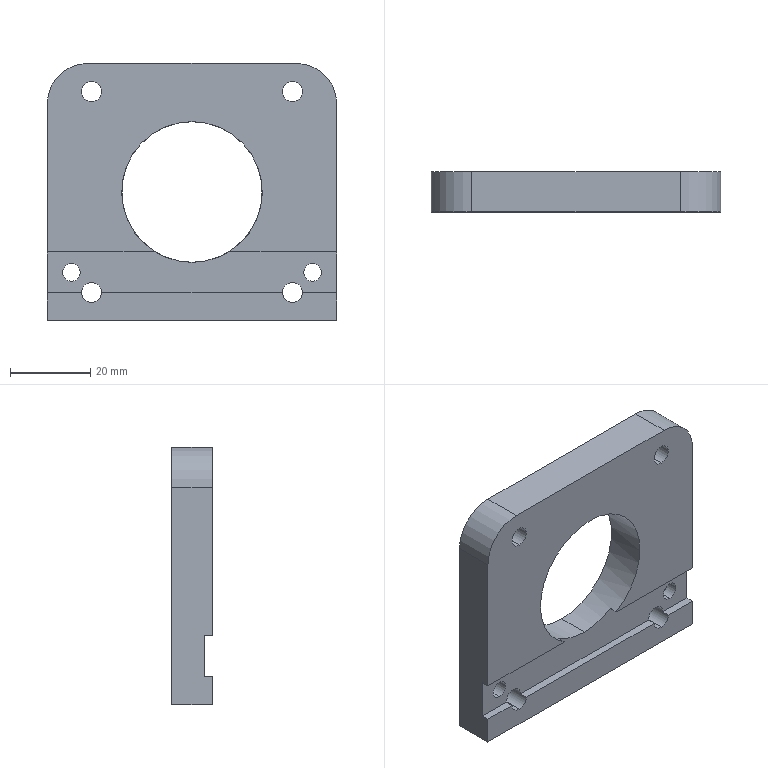Part | SolidWorks | features HoleWzd 5, ICE 5, Fillet 2, Extrusion 1 | 1 solid | 35 faces | box 72 x 10 x 64 mm | volume 33293 mm3 | cylinder 20 | plane 15 | commonest cylinder face diameters 5 x8 4.4 x4 8 x4 20 x2 35 x2
STEP:
#1=CARTESIAN_POINT('',(26.5,0.,40.5));
#2=VERTEX_POINT('',#1);
#3=CARTESIAN_POINT('',(24.001,0.,42.925));
#4=VERTEX_POINT('',#3);
#5=CARTESIAN_POINT('',(26.5,0.,43.));
#6=DIRECTION('',(0.,1.,0.));
#7=DIRECTION('',(0.,0.,1.));
#8=AXIS2_PLACEMENT_3D('',#5,#6,#7);
#9=CIRCLE('',#8,2.5);
#10=EDGE_CURVE('',#2,#4,#9,.T.);
#11=ORIENTED_EDGE('',*,*,#10,.F.);
#12=CARTESIAN_POINT('',(26.5,10.,40.5));
#13=VERTEX_POINT('',#12);
#14=CARTESIAN_POINT('',(26.5,10.,40.5));
#15=DIRECTION('',(0.,1.,0.));
#16=VECTOR('',#15,1000.);
#17=LINE('',#14,#16);
#18=EDGE_CURVE('',#2,#13,#17,.T.);
#19=ORIENTED_EDGE('',*,*,#18,.T.);
#20=CARTESIAN_POINT('',(26.5,10.,45.5));
#21=VERTEX_POINT('',#20);
#22=CARTESIAN_POINT('',(26.5,10.,43.));
#23=DIRECTION('',(0.,1.,0.));
#24=DIRECTION('',(0.,0.,1.));
#25=AXIS2_PLACEMENT_3D('',#22,#23,#24);
#26=CIRCLE('',#25,2.5);
#27=EDGE_CURVE('',#13,#21,#26,.T.);
#28=ORIENTED_EDGE('',*,*,#27,.T.);
#29=CARTESIAN_POINT('',(26.5,2.,45.5));
#30=VERTEX_POINT('',#29);
#31=CARTESIAN_POINT('',(26.5,10.,45.5));
#32=DIRECTION('',(0.,1.,0.));
#33=VECTOR('',#32,1000.);
#34=LINE('',#31,#33);
#35=EDGE_CURVE('',#30,#21,#34,.T.);
#36=ORIENTED_EDGE('',*,*,#35,.F.);
#37=CARTESIAN_POINT('',(24.001,2.,42.925));
#38=VERTEX_POINT('',#37);
#39=CARTESIAN_POINT('',(26.5,2.,43.));
#40=DIRECTION('',(0.,1.,0.));
#41=DIRECTION('',(0.,0.,-1.));
#42=AXIS2_PLACEMENT_3D('',#39,#40,#41);
#43=CIRCLE('',#42,2.5);
#44=EDGE_CURVE('',#38,#30,#43,.T.);
#45=ORIENTED_EDGE('',*,*,#44,.F.);
#46=CARTESIAN_POINT('',(24.001,10.,42.925));
#47=DIRECTION('',(0.,-1.,0.));
#48=VECTOR('',#47,1000.);
#49=LINE('',#46,#48);
#50=EDGE_CURVE('',#38,#4,#49,.T.);
#51=ORIENTED_EDGE('',*,*,#50,.T.);
#52=EDGE_LOOP('',(#11,#19,#28,#36,#45,#51));
#53=FACE_OUTER_BOUND('',#52,.T.);
#54=CARTESIAN_POINT('',(26.5,10.,43.));
#55=DIRECTION('',(0.,1.,0.));
#56=DIRECTION('',(0.,0.,1.));
#57=AXIS2_PLACEMENT_3D('',#54,#55,#56);
#58=CYLINDRICAL_SURFACE('',#57,2.5);
#59=ADVANCED_FACE('',(#53),#58,.F.);
#60=CARTESIAN_POINT('',(26.5,0.,90.5));
#61=VERTEX_POINT('',#60);
#62=CARTESIAN_POINT('',(26.5,0.,95.5));
#63=VERTEX_POINT('',#62);
#64=CARTESIAN_POINT('',(26.5,0.,93.));
#65=DIRECTION('',(0.,1.,0.));
#66=DIRECTION('',(0.,0.,1.));
#67=AXIS2_PLACEMENT_3D('',#64,#65,#66);
#68=CIRCLE('',#67,2.5);
#69=EDGE_CURVE('',#61,#63,#68,.T.);
#70=ORIENTED_EDGE('',*,*,#69,.F.);
#71=CARTESIAN_POINT('',(26.5,10.,90.5));
#72=VERTEX_POINT('',#71);
#73=CARTESIAN_POINT('',(26.5,10.,90.5));
#74=DIRECTION('',(0.,1.,0.));
#75=VECTOR('',#74,1000.);
#76=LINE('',#73,#75);
#77=EDGE_CURVE('',#61,#72,#76,.T.);
#78=ORIENTED_EDGE('',*,*,#77,.T.);
#79=CARTESIAN_POINT('',(26.5,10.,95.5));
#80=VERTEX_POINT('',#79);
#81=CARTESIAN_POINT('',(26.5,10.,93.));
#82=DIRECTION('',(0.,1.,0.));
#83=DIRECTION('',(0.,0.,1.));
#84=AXIS2_PLACEMENT_3D('',#81,#82,#83);
#85=CIRCLE('',#84,2.5);
#86=EDGE_CURVE('',#72,#80,#85,.T.);
#87=ORIENTED_EDGE('',*,*,#86,.T.);
#88=CARTESIAN_POINT('',(26.5,10.,95.5));
#89=DIRECTION('',(0.,1.,0.));
#90=VECTOR('',#89,1000.);
#91=LINE('',#88,#90);
#92=EDGE_CURVE('',#63,#80,#91,.T.);
#93=ORIENTED_EDGE('',*,*,#92,.F.);
#94=EDGE_LOOP('',(#70,#78,#87,#93));
#95=FACE_OUTER_BOUND('',#94,.T.);
#96=CARTESIAN_POINT('',(26.5,10.,93.));
#97=DIRECTION('',(0.,1.,0.));
#98=DIRECTION('',(0.,0.,1.));
#99=AXIS2_PLACEMENT_3D('',#96,#97,#98);
#100=CYLINDRICAL_SURFACE('',#99,2.5);
#101=ADVANCED_FACE('',(#95),#100,.F.);
#102=CARTESIAN_POINT('',(76.5,0.,90.5));
#103=VERTEX_POINT('',#102);
#104=CARTESIAN_POINT('',(76.5,0.,95.5));
#105=VERTEX_POINT('',#104);
#106=CARTESIAN_POINT('',(76.5,0.,93.));
#107=DIRECTION('',(0.,1.,0.));
#108=DIRECTION('',(0.,0.,1.));
#109=AXIS2_PLACEMENT_3D('',#106,#107,#108);
#110=CIRCLE('',#109,2.5);
#111=EDGE_CURVE('',#103,#105,#110,.T.);
#112=ORIENTED_EDGE('',*,*,#111,.F.);
#113=CARTESIAN_POINT('',(76.5,10.,90.5));
#114=VERTEX_POINT('',#113);
#115=CARTESIAN_POINT('',(76.5,10.,90.5));
#116=DIRECTION('',(0.,1.,0.));
#117=VECTOR('',#116,1000.);
#118=LINE('',#115,#117);
#119=EDGE_CURVE('',#103,#114,#118,.T.);
#120=ORIENTED_EDGE('',*,*,#119,.T.);
#121=CARTESIAN_POINT('',(76.5,10.,95.5));
#122=VERTEX_POINT('',#121);
#123=CARTESIAN_POINT('',(76.5,10.,93.));
#124=DIRECTION('',(0.,1.,0.));
#125=DIRECTION('',(0.,0.,1.));
#126=AXIS2_PLACEMENT_3D('',#123,#124,#125);
#127=CIRCLE('',#126,2.5);
#128=EDGE_CURVE('',#114,#122,#127,.T.);
#129=ORIENTED_EDGE('',*,*,#128,.T.);
#130=CARTESIAN_POINT('',(76.5,10.,95.5));
#131=DIRECTION('',(0.,1.,0.));
#132=VECTOR('',#131,1000.);
#133=LINE('',#130,#132);
#134=EDGE_CURVE('',#105,#122,#133,.T.);
#135=ORIENTED_EDGE('',*,*,#134,.F.);
#136=EDGE_LOOP('',(#112,#120,#129,#135));
#137=FACE_OUTER_BOUND('',#136,.T.);
#138=CARTESIAN_POINT('',(76.5,10.,93.));
#139=DIRECTION('',(0.,1.,0.));
#140=DIRECTION('',(0.,0.,1.));
#141=AXIS2_PLACEMENT_3D('',#138,#139,#140);
#142=CYLINDRICAL_SURFACE('',#141,2.5);
#143=ADVANCED_FACE('',(#137),#142,.F.);
#144=CARTESIAN_POINT('',(76.5,0.,40.5));
#145=VERTEX_POINT('',#144);
#146=CARTESIAN_POINT('',(74.001,0.,42.925));
#147=VERTEX_POINT('',#146);
#148=CARTESIAN_POINT('',(76.5,0.,43.));
#149=DIRECTION('',(0.,1.,0.));
#150=DIRECTION('',(0.,0.,1.));
#151=AXIS2_PLACEMENT_3D('',#148,#149,#150);
#152=CIRCLE('',#151,2.5);
#153=EDGE_CURVE('',#145,#147,#152,.T.);
#154=ORIENTED_EDGE('',*,*,#153,.F.);
#155=CARTESIAN_POINT('',(76.5,10.,40.5));
#156=VERTEX_POINT('',#155);
#157=CARTESIAN_POINT('',(76.5,10.,40.5));
#158=DIRECTION('',(0.,1.,0.));
#159=VECTOR('',#158,1000.);
#160=LINE('',#157,#159);
#161=EDGE_CURVE('',#145,#156,#160,.T.);
#162=ORIENTED_EDGE('',*,*,#161,.T.);
#163=CARTESIAN_POINT('',(76.5,10.,45.5));
#164=VERTEX_POINT('',#163);
#165=CARTESIAN_POINT('',(76.5,10.,43.));
#166=DIRECTION('',(0.,1.,0.));
#167=DIRECTION('',(0.,0.,1.));
#168=AXIS2_PLACEMENT_3D('',#165,#166,#167);
#169=CIRCLE('',#168,2.5);
#170=EDGE_CURVE('',#156,#164,#169,.T.);
#171=ORIENTED_EDGE('',*,*,#170,.T.);
#172=CARTESIAN_POINT('',(76.5,2.,45.5));
#173=VERTEX_POINT('',#172);
#174=CARTESIAN_POINT('',(76.5,10.,45.5));
#175=DIRECTION('',(0.,1.,0.));
#176=VECTOR('',#175,1000.);
#177=LINE('',#174,#176);
#178=EDGE_CURVE('',#173,#164,#177,.T.);
#179=ORIENTED_EDGE('',*,*,#178,.F.);
#180=CARTESIAN_POINT('',(74.001,2.,42.925));
#181=VERTEX_POINT('',#180);
#182=CARTESIAN_POINT('',(76.5,2.,43.));
#183=DIRECTION('',(0.,1.,0.));
#184=DIRECTION('',(0.,0.,-1.));
#185=AXIS2_PLACEMENT_3D('',#182,#183,#184);
#186=CIRCLE('',#185,2.5);
#187=EDGE_CURVE('',#181,#173,#186,.T.);
#188=ORIENTED_EDGE('',*,*,#187,.F.);
#189=CARTESIAN_POINT('',(74.001,10.,42.925));
#190=DIRECTION('',(0.,-1.,0.));
#191=VECTOR('',#190,1000.);
#192=LINE('',#189,#191);
#193=EDGE_CURVE('',#181,#147,#192,.T.);
#194=ORIENTED_EDGE('',*,*,#193,.T.);
#195=EDGE_LOOP('',(#154,#162,#171,#179,#188,#194));
#196=FACE_OUTER_BOUND('',#195,.T.);
#197=CARTESIAN_POINT('',(76.5,10.,43.));
#198=DIRECTION('',(0.,1.,0.));
#199=DIRECTION('',(0.,0.,1.));
#200=AXIS2_PLACEMENT_3D('',#197,#198,#199);
#201=CYLINDRICAL_SURFACE('',#200,2.5);
#202=ADVANCED_FACE('',(#196),#201,.F.);
#203=CARTESIAN_POINT('',(21.5,5.,44.));
#204=VERTEX_POINT('',#203);
#205=CARTESIAN_POINT('',(21.5,5.,52.));
#206=VERTEX_POINT('',#205);
#207=CARTESIAN_POINT('',(21.5,5.,48.));
#208=DIRECTION('',(0.,1.,0.));
#209=DIRECTION('',(0.,0.,1.));
#210=AXIS2_PLACEMENT_3D('',#207,#208,#209);
#211=CIRCLE('',#210,4.);
#212=EDGE_CURVE('',#204,#206,#211,.T.);
#213=ORIENTED_EDGE('',*,*,#212,.F.);
#214=CARTESIAN_POINT('',(21.5,10.,44.));
#215=VERTEX_POINT('',#214);
#216=CARTESIAN_POINT('',(21.5,10.,44.));
#217=DIRECTION('',(0.,1.,0.));
#218=VECTOR('',#217,1000.);
#219=LINE('',#216,#218);
#220=EDGE_CURVE('',#204,#215,#219,.T.);
#221=ORIENTED_EDGE('',*,*,#220,.T.);
#222=CARTESIAN_POINT('',(21.5,10.,52.));
#223=VERTEX_POINT('',#222);
#224=CARTESIAN_POINT('',(21.5,10.,48.));
#225=DIRECTION('',(0.,1.,0.));
#226=DIRECTION('',(0.,0.,1.));
#227=AXIS2_PLACEMENT_3D('',#224,#225,#226);
#228=CIRCLE('',#227,4.);
#229=EDGE_CURVE('',#215,#223,#228,.T.);
#230=ORIENTED_EDGE('',*,*,#229,.T.);
#231=CARTESIAN_POINT('',(21.5,10.,52.));
#232=DIRECTION('',(0.,1.,0.));
#233=VECTOR('',#232,1000.);
#234=LINE('',#231,#233);
#235=EDGE_CURVE('',#206,#223,#234,.T.);
#236=ORIENTED_EDGE('',*,*,#235,.F.);
#237=EDGE_LOOP('',(#213,#221,#230,#236));
#238=FACE_OUTER_BOUND('',#237,.T.);
#239=CARTESIAN_POINT('',(21.5,10.,48.));
#240=DIRECTION('',(0.,1.,0.));
#241=DIRECTION('',(0.,0.,1.));
#242=AXIS2_PLACEMENT_3D('',#239,#240,#241);
#243=CYLINDRICAL_SURFACE('',#242,4.);
#244=ADVANCED_FACE('',(#238),#243,.F.);
#245=CARTESIAN_POINT('',(81.5,5.,44.));
#246=VERTEX_POINT('',#245);
#247=CARTESIAN_POINT('',(81.5,5.,52.));
#248=VERTEX_POINT('',#247);
#249=CARTESIAN_POINT('',(81.5,5.,48.));
#250=DIRECTION('',(0.,1.,0.));
#251=DIRECTION('',(0.,0.,1.));
#252=AXIS2_PLACEMENT_3D('',#249,#250,#251);
#253=CIRCLE('',#252,4.);
#254=EDGE_CURVE('',#246,#248,#253,.T.);
#255=ORIENTED_EDGE('',*,*,#254,.F.);
#256=CARTESIAN_POINT('',(81.5,10.,44.));
#257=VERTEX_POINT('',#256);
#258=CARTESIAN_POINT('',(81.5,10.,44.));
#259=DIRECTION('',(0.,1.,0.));
#260=VECTOR('',#259,1000.);
#261=LINE('',#258,#260);
#262=EDGE_CURVE('',#246,#257,#261,.T.);
#263=ORIENTED_EDGE('',*,*,#262,.T.);
#264=CARTESIAN_POINT('',(81.5,10.,52.));
#265=VERTEX_POINT('',#264);
#266=CARTESIAN_POINT('',(81.5,10.,48.));
#267=DIRECTION('',(0.,1.,0.));
#268=DIRECTION('',(0.,0.,1.));
#269=AXIS2_PLACEMENT_3D('',#266,#267,#268);
#270=CIRCLE('',#269,4.);
#271=EDGE_CURVE('',#257,#265,#270,.T.);
#272=ORIENTED_EDGE('',*,*,#271,.T.);
#273=CARTESIAN_POINT('',(81.5,10.,52.));
#274=DIRECTION('',(0.,1.,0.));
#275=VECTOR('',#274,1000.);
#276=LINE('',#273,#275);
#277=EDGE_CURVE('',#248,#265,#276,.T.);
#278=ORIENTED_EDGE('',*,*,#277,.F.);
#279=EDGE_LOOP('',(#255,#263,#272,#278));
#280=FACE_OUTER_BOUND('',#279,.T.);
#281=CARTESIAN_POINT('',(81.5,10.,48.));
#282=DIRECTION('',(0.,1.,0.));
#283=DIRECTION('',(0.,0.,1.));
#284=AXIS2_PLACEMENT_3D('',#281,#282,#283);
#285=CYLINDRICAL_SURFACE('',#284,4.);
#286=ADVANCED_FACE('',(#280),#285,.F.);
#287=CARTESIAN_POINT('',(51.5,2.,50.5));
#288=VERTEX_POINT('',#287);
#289=CARTESIAN_POINT('',(42.362,2.,53.075));
#290=VERTEX_POINT('',#289);
#291=CARTESIAN_POINT('',(51.5,2.,68.));
#292=DIRECTION('',(0.,1.,0.));
#293=DIRECTION('',(0.,0.,-1.));
#294=AXIS2_PLACEMENT_3D('',#291,#292,#293);
#295=CIRCLE('',#294,17.5);
#296=EDGE_CURVE('',#288,#290,#295,.T.);
#297=ORIENTED_EDGE('',*,*,#296,.F.);
#298=CARTESIAN_POINT('',(51.5,10.,50.5));
#299=VERTEX_POINT('',#298);
#300=CARTESIAN_POINT('',(51.5,0.,50.5));
#301=DIRECTION('',(0.,1.,0.));
#302=VECTOR('',#301,1000.);
#303=LINE('',#300,#302);
#304=EDGE_CURVE('',#288,#299,#303,.T.);
#305=ORIENTED_EDGE('',*,*,#304,.T.);
#306=CARTESIAN_POINT('',(51.5,10.,85.5));
#307=VERTEX_POINT('',#306);
#308=CARTESIAN_POINT('',(51.5,10.,68.));
#309=DIRECTION('',(0.,1.,0.));
#310=DIRECTION('',(0.,0.,1.));
#311=AXIS2_PLACEMENT_3D('',#308,#309,#310);
#312=CIRCLE('',#311,17.5);
#313=EDGE_CURVE('',#299,#307,#312,.T.);
#314=ORIENTED_EDGE('',*,*,#313,.T.);
#315=CARTESIAN_POINT('',(51.5,0.,85.5));
#316=VERTEX_POINT('',#315);
#317=CARTESIAN_POINT('',(51.5,0.,85.5));
#318=DIRECTION('',(0.,1.,0.));
#319=VECTOR('',#318,1000.);
#320=LINE('',#317,#319);
#321=EDGE_CURVE('',#316,#307,#320,.T.);
#322=ORIENTED_EDGE('',*,*,#321,.F.);
#323=CARTESIAN_POINT('',(42.362,0.,53.075));
#324=VERTEX_POINT('',#323);
#325=CARTESIAN_POINT('',(51.5,0.,68.));
#326=DIRECTION('',(0.,1.,0.));
#327=DIRECTION('',(0.,0.,1.));
#328=AXIS2_PLACEMENT_3D('',#325,#326,#327);
#329=CIRCLE('',#328,17.5);
#330=EDGE_CURVE('',#324,#316,#329,.T.);
#331=ORIENTED_EDGE('',*,*,#330,.F.);
#332=CARTESIAN_POINT('',(42.362,0.,53.075));
#333=DIRECTION('',(0.,1.,0.));
#334=VECTOR('',#333,1000.);
#335=LINE('',#332,#334);
#336=EDGE_CURVE('',#324,#290,#335,.T.);
#337=ORIENTED_EDGE('',*,*,#336,.T.);
#338=EDGE_LOOP('',(#297,#305,#314,#322,#331,#337));
#339=FACE_OUTER_BOUND('',#338,.T.);
#340=CARTESIAN_POINT('',(51.5,0.,68.));
#341=DIRECTION('',(0.,1.,0.));
#342=DIRECTION('',(0.,0.,1.));
#343=AXIS2_PLACEMENT_3D('',#340,#341,#342);
#344=CYLINDRICAL_SURFACE('',#343,17.5);
#345=ADVANCED_FACE('',(#339),#344,.F.);
#346=CARTESIAN_POINT('',(21.5,2.,45.8));
#347=VERTEX_POINT('',#346);
#348=CARTESIAN_POINT('',(21.5,2.,50.2));
#349=VERTEX_POINT('',#348);
#350=CARTESIAN_POINT('',(21.5,2.,48.));
#351=DIRECTION('',(0.,1.,0.));
#352=DIRECTION('',(0.,0.,-1.));
#353=AXIS2_PLACEMENT_3D('',#350,#351,#352);
#354=CIRCLE('',#353,2.2);
#355=EDGE_CURVE('',#347,#349,#354,.T.);
#356=ORIENTED_EDGE('',*,*,#355,.F.);
#357=CARTESIAN_POINT('',(21.5,5.,45.8));
#358=VERTEX_POINT('',#357);
#359=CARTESIAN_POINT('',(21.5,10.,45.8));
#360=DIRECTION('',(0.,1.,0.));
#361=VECTOR('',#360,1000.);
#362=LINE('',#359,#361);
#363=EDGE_CURVE('',#347,#358,#362,.T.);
#364=ORIENTED_EDGE('',*,*,#363,.T.);
#365=CARTESIAN_POINT('',(21.5,5.,50.2));
#366=VERTEX_POINT('',#365);
#367=CARTESIAN_POINT('',(21.5,5.,48.));
#368=DIRECTION('',(0.,1.,0.));
#369=DIRECTION('',(0.,0.,1.));
#370=AXIS2_PLACEMENT_3D('',#367,#368,#369);
#371=CIRCLE('',#370,2.2);
#372=EDGE_CURVE('',#358,#366,#371,.T.);
#373=ORIENTED_EDGE('',*,*,#372,.T.);
#374=CARTESIAN_POINT('',(21.5,10.,50.2));
#375=DIRECTION('',(0.,1.,0.));
#376=VECTOR('',#375,1000.);
#377=LINE('',#374,#376);
#378=EDGE_CURVE('',#349,#366,#377,.T.);
#379=ORIENTED_EDGE('',*,*,#378,.F.);
#380=EDGE_LOOP('',(#356,#364,#373,#379));
#381=FACE_OUTER_BOUND('',#380,.T.);
#382=CARTESIAN_POINT('',(21.5,10.,48.));
#383=DIRECTION('',(0.,1.,0.));
#384=DIRECTION('',(0.,0.,1.));
#385=AXIS2_PLACEMENT_3D('',#382,#383,#384);
#386=CYLINDRICAL_SURFACE('',#385,2.2);
#387=ADVANCED_FACE('',(#381),#386,.F.);
#388=CARTESIAN_POINT('',(81.5,2.,45.8));
#389=VERTEX_POINT('',#388);
#390=CARTESIAN_POINT('',(81.5,2.,50.2));
#391=VERTEX_POINT('',#390);
#392=CARTESIAN_POINT('',(81.5,2.,48.));
#393=DIRECTION('',(0.,1.,0.));
#394=DIRECTION('',(0.,0.,-1.));
#395=AXIS2_PLACEMENT_3D('',#392,#393,#394);
#396=CIRCLE('',#395,2.2);
#397=EDGE_CURVE('',#389,#391,#396,.T.);
#398=ORIENTED_EDGE('',*,*,#397,.F.);
#399=CARTESIAN_POINT('',(81.5,5.,45.8));
#400=VERTEX_POINT('',#399);
#401=CARTESIAN_POINT('',(81.5,10.,45.8));
#402=DIRECTION('',(0.,1.,0.));
#403=VECTOR('',#402,1000.);
#404=LINE('',#401,#403);
#405=EDGE_CURVE('',#389,#400,#404,.T.);
#406=ORIENTED_EDGE('',*,*,#405,.T.);
#407=CARTESIAN_POINT('',(81.5,5.,50.2));
#408=VERTEX_POINT('',#407);
#409=CARTESIAN_POINT('',(81.5,5.,48.));
#410=DIRECTION('',(0.,1.,0.));
#411=DIRECTION('',(0.,0.,1.));
#412=AXIS2_PLACEMENT_3D('',#409,#410,#411);
#413=CIRCLE('',#412,2.2);
#414=EDGE_CURVE('',#400,#408,#413,.T.);
#415=ORIENTED_EDGE('',*,*,#414,.T.);
#416=CARTESIAN_POINT('',(81.5,10.,50.2));
#417=DIRECTION('',(0.,1.,0.));
#418=VECTOR('',#417,1000.);
#419=LINE('',#416,#418);
#420=EDGE_CURVE('',#391,#408,#419,.T.);
#421=ORIENTED_EDGE('',*,*,#420,.F.);
#422=EDGE_LOOP('',(#398,#406,#415,#421));
#423=FACE_OUTER_BOUND('',#422,.T.);
#424=CARTESIAN_POINT('',(81.5,10.,48.));
#425=DIRECTION('',(0.,1.,0.));
#426=DIRECTION('',(0.,0.,1.));
#427=AXIS2_PLACEMENT_3D('',#424,#425,#426);
#428=CYLINDRICAL_SURFACE('',#427,2.2);
#429=ADVANCED_FACE('',(#423),#428,.F.);
#430=CARTESIAN_POINT('',(15.5,0.,42.925));
#431=VERTEX_POINT('',#430);
#432=CARTESIAN_POINT('',(-50.34,0.,42.925));
#433=DIRECTION('',(1.,0.,0.));
#434=VECTOR('',#433,1000.);
#435=LINE('',#432,#434);
#436=EDGE_CURVE('',#431,#4,#435,.T.);
#437=ORIENTED_EDGE('',*,*,#436,.F.);
#438=CARTESIAN_POINT('',(15.5,0.,36.));
#439=VERTEX_POINT('',#438);
#440=CARTESIAN_POINT('',(15.5,0.,100.));
#441=DIRECTION('',(0.,0.,-1.));
#442=VECTOR('',#441,1000.);
#443=LINE('',#440,#442);
#444=EDGE_CURVE('',#431,#439,#443,.T.);
#445=ORIENTED_EDGE('',*,*,#444,.T.);
#446=CARTESIAN_POINT('',(87.5,0.,36.));
#447=VERTEX_POINT('',#446);
#448=CARTESIAN_POINT('',(0.,0.,36.));
#449=DIRECTION('',(-1.,0.,0.));
#450=VECTOR('',#449,1000.);
#451=LINE('',#448,#450);
#452=EDGE_CURVE('',#447,#439,#451,.T.);
#453=ORIENTED_EDGE('',*,*,#452,.F.);
#454=CARTESIAN_POINT('',(87.5,0.,42.925));
#455=VERTEX_POINT('',#454);
#456=CARTESIAN_POINT('',(87.5,0.,100.));
#457=DIRECTION('',(0.,0.,1.));
#458=VECTOR('',#457,1000.);
#459=LINE('',#456,#458);
#460=EDGE_CURVE('',#447,#455,#459,.T.);
#461=ORIENTED_EDGE('',*,*,#460,.T.);
#462=CARTESIAN_POINT('',(78.999,0.,42.925));
#463=VERTEX_POINT('',#462);
#464=CARTESIAN_POINT('',(-50.34,0.,42.925));
#465=DIRECTION('',(1.,0.,0.));
#466=VECTOR('',#465,1000.);
#467=LINE('',#464,#466);
#468=EDGE_CURVE('',#463,#455,#467,.T.);
#469=ORIENTED_EDGE('',*,*,#468,.F.);
#470=CARTESIAN_POINT('',(76.5,0.,43.));
#471=DIRECTION('',(0.,1.,0.));
#472=DIRECTION('',(0.,0.,1.));
#473=AXIS2_PLACEMENT_3D('',#470,#471,#472);
#474=CIRCLE('',#473,2.5);
#475=EDGE_CURVE('',#463,#145,#474,.T.);
#476=ORIENTED_EDGE('',*,*,#475,.T.);
#477=ORIENTED_EDGE('',*,*,#153,.T.);
#478=CARTESIAN_POINT('',(28.999,0.,42.925));
#479=VERTEX_POINT('',#478);
#480=CARTESIAN_POINT('',(-50.34,0.,42.925));
#481=DIRECTION('',(1.,0.,0.));
#482=VECTOR('',#481,1000.);
#483=LINE('',#480,#482);
#484=EDGE_CURVE('',#479,#147,#483,.T.);
#485=ORIENTED_EDGE('',*,*,#484,.F.);
#486=CARTESIAN_POINT('',(26.5,0.,43.));
#487=DIRECTION('',(0.,1.,0.));
#488=DIRECTION('',(0.,0.,1.));
#489=AXIS2_PLACEMENT_3D('',#486,#487,#488);
#490=CIRCLE('',#489,2.5);
#491=EDGE_CURVE('',#479,#2,#490,.T.);
#492=ORIENTED_EDGE('',*,*,#491,.T.);
#493=ORIENTED_EDGE('',*,*,#10,.T.);
#494=EDGE_LOOP('',(#437,#445,#453,#461,#469,#476,#477,#485,#492,#493));
#495=FACE_OUTER_BOUND('',#494,.T.);
#496=CARTESIAN_POINT('',(0.,0.,0.));
#497=DIRECTION('',(0.,-1.,0.));
#498=DIRECTION('',(0.,0.,-1.));
#499=AXIS2_PLACEMENT_3D('',#496,#497,#498);
#500=PLANE('',#499);
#501=ADVANCED_FACE('',(#495),#500,.T.);
#502=ORIENTED_EDGE('',*,*,#405,.F.);
#503=CARTESIAN_POINT('',(81.5,2.,48.));
#504=DIRECTION('',(0.,1.,0.));
#505=DIRECTION('',(0.,0.,-1.));
#506=AXIS2_PLACEMENT_3D('',#503,#504,#505);
#507=CIRCLE('',#506,2.2);
#508=EDGE_CURVE('',#391,#389,#507,.T.);
#509=ORIENTED_EDGE('',*,*,#508,.F.);
#510=ORIENTED_EDGE('',*,*,#420,.T.);
#511=CARTESIAN_POINT('',(81.5,5.,48.));
#512=DIRECTION('',(0.,1.,0.));
#513=DIRECTION('',(0.,0.,1.));
#514=AXIS2_PLACEMENT_3D('',#511,#512,#513);
#515=CIRCLE('',#514,2.2);
#516=EDGE_CURVE('',#408,#400,#515,.T.);
#517=ORIENTED_EDGE('',*,*,#516,.T.);
#518=EDGE_LOOP('',(#502,#509,#510,#517));
#519=FACE_OUTER_BOUND('',#518,.T.);
#520=CARTESIAN_POINT('',(81.5,10.,48.));
#521=DIRECTION('',(0.,1.,0.));
#522=DIRECTION('',(0.,0.,1.));
#523=AXIS2_PLACEMENT_3D('',#520,#521,#522);
#524=CYLINDRICAL_SURFACE('',#523,2.2);
#525=ADVANCED_FACE('',(#519),#524,.F.);
#526=ORIENTED_EDGE('',*,*,#363,.F.);
#527=CARTESIAN_POINT('',(21.5,2.,48.));
#528=DIRECTION('',(0.,1.,0.));
#529=DIRECTION('',(0.,0.,-1.));
#530=AXIS2_PLACEMENT_3D('',#527,#528,#529);
#531=CIRCLE('',#530,2.2);
#532=EDGE_CURVE('',#349,#347,#531,.T.);
#533=ORIENTED_EDGE('',*,*,#532,.F.);
#534=ORIENTED_EDGE('',*,*,#378,.T.);
#535=CARTESIAN_POINT('',(21.5,5.,48.));
#536=DIRECTION('',(0.,1.,0.));
#537=DIRECTION('',(0.,0.,1.));
#538=AXIS2_PLACEMENT_3D('',#535,#536,#537);
#539=CIRCLE('',#538,2.2);
#540=EDGE_CURVE('',#366,#358,#539,.T.);
#541=ORIENTED_EDGE('',*,*,#540,.T.);
#542=EDGE_LOOP('',(#526,#533,#534,#541));
#543=FACE_OUTER_BOUND('',#542,.T.);
#544=CARTESIAN_POINT('',(21.5,10.,48.));
#545=DIRECTION('',(0.,1.,0.));
#546=DIRECTION('',(0.,0.,1.));
#547=AXIS2_PLACEMENT_3D('',#544,#545,#546);
#548=CYLINDRICAL_SURFACE('',#547,2.2);
#549=ADVANCED_FACE('',(#543),#548,.F.);
#550=CARTESIAN_POINT('',(25.5,10.,100.));
#551=VERTEX_POINT('',#550);
#552=CARTESIAN_POINT('',(77.5,10.,100.));
#553=VERTEX_POINT('',#552);
#554=CARTESIAN_POINT('',(103.,10.,100.));
#555=DIRECTION('',(1.,0.,0.));
#556=VECTOR('',#555,1000.);
#557=LINE('',#554,#556);
#558=EDGE_CURVE('',#551,#553,#557,.T.);
#559=ORIENTED_EDGE('',*,*,#558,.F.);
#560=CARTESIAN_POINT('',(25.5,0.,100.));
#561=VERTEX_POINT('',#560);
#562=CARTESIAN_POINT('',(25.5,10.,100.));
#563=DIRECTION('',(0.,-1.,0.));
#564=VECTOR('',#563,1000.);
#565=LINE('',#562,#564);
#566=EDGE_CURVE('',#551,#561,#565,.T.);
#567=ORIENTED_EDGE('',*,*,#566,.T.);
#568=CARTESIAN_POINT('',(77.5,0.,100.));
#569=VERTEX_POINT('',#568);
#570=CARTESIAN_POINT('',(103.,0.,100.));
#571=DIRECTION('',(1.,0.,0.));
#572=VECTOR('',#571,1000.);
#573=LINE('',#570,#572);
#574=EDGE_CURVE('',#561,#569,#573,.T.);
#575=ORIENTED_EDGE('',*,*,#574,.T.);
#576=CARTESIAN_POINT('',(77.5,10.,100.));
#577=DIRECTION('',(0.,1.,0.));
#578=VECTOR('',#577,1000.);
#579=LINE('',#576,#578);
#580=EDGE_CURVE('',#569,#553,#579,.T.);
#581=ORIENTED_EDGE('',*,*,#580,.T.);
#582=EDGE_LOOP('',(#559,#567,#575,#581));
#583=FACE_OUTER_BOUND('',#582,.T.);
#584=CARTESIAN_POINT('',(103.,10.,100.));
#585=DIRECTION('',(0.,0.,-1.));
#586=DIRECTION('',(-1.,0.,0.));
#587=AXIS2_PLACEMENT_3D('',#584,#585,#586);
#588=PLANE('',#587);
#589=ADVANCED_FACE('',(#583),#588,.F.);
#590=CARTESIAN_POINT('',(26.5,10.,43.));
#591=DIRECTION('',(0.,1.,0.));
#592=DIRECTION('',(0.,0.,1.));
#593=AXIS2_PLACEMENT_3D('',#590,#591,#592);
#594=CIRCLE('',#593,2.5);
#595=EDGE_CURVE('',#21,#13,#594,.T.);
#596=ORIENTED_EDGE('',*,*,#595,.F.);
#597=ORIENTED_EDGE('',*,*,#27,.F.);
#598=EDGE_LOOP('',(#596,#597));
#599=FACE_BOUND('',#598,.T.);
#600=CARTESIAN_POINT('',(26.5,10.,93.));
#601=DIRECTION('',(0.,1.,0.));
#602=DIRECTION('',(0.,0.,1.));
#603=AXIS2_PLACEMENT_3D('',#600,#601,#602);
#604=CIRCLE('',#603,2.5);
#605=EDGE_CURVE('',#80,#72,#604,.T.);
#606=ORIENTED_EDGE('',*,*,#605,.F.);
#607=ORIENTED_EDGE('',*,*,#86,.F.);
#608=EDGE_LOOP('',(#606,#607));
#609=FACE_BOUND('',#608,.T.);
#610=CARTESIAN_POINT('',(76.5,10.,93.));
#611=DIRECTION('',(0.,1.,0.));
#612=DIRECTION('',(0.,0.,1.));
#613=AXIS2_PLACEMENT_3D('',#610,#611,#612);
#614=CIRCLE('',#613,2.5);
#615=EDGE_CURVE('',#122,#114,#614,.T.);
#616=ORIENTED_EDGE('',*,*,#615,.F.);
#617=ORIENTED_EDGE('',*,*,#128,.F.);
#618=EDGE_LOOP('',(#616,#617));
#619=FACE_BOUND('',#618,.T.);
#620=CARTESIAN_POINT('',(76.5,10.,43.));
#621=DIRECTION('',(0.,1.,0.));
#622=DIRECTION('',(0.,0.,1.));
#623=AXIS2_PLACEMENT_3D('',#620,#621,#622);
#624=CIRCLE('',#623,2.5);
#625=EDGE_CURVE('',#164,#156,#624,.T.);
#626=ORIENTED_EDGE('',*,*,#625,.F.);
#627=ORIENTED_EDGE('',*,*,#170,.F.);
#628=EDGE_LOOP('',(#626,#627));
#629=FACE_BOUND('',#628,.T.);
#630=CARTESIAN_POINT('',(21.5,10.,48.));
#631=DIRECTION('',(0.,1.,0.));
#632=DIRECTION('',(0.,0.,1.));
#633=AXIS2_PLACEMENT_3D('',#630,#631,#632);
#634=CIRCLE('',#633,4.);
#635=EDGE_CURVE('',#223,#215,#634,.T.);
#636=ORIENTED_EDGE('',*,*,#635,.F.);
#637=ORIENTED_EDGE('',*,*,#229,.F.);
#638=EDGE_LOOP('',(#636,#637));
#639=FACE_BOUND('',#638,.T.);
#640=CARTESIAN_POINT('',(81.5,10.,48.));
#641=DIRECTION('',(0.,1.,0.));
#642=DIRECTION('',(0.,0.,1.));
#643=AXIS2_PLACEMENT_3D('',#640,#641,#642);
#644=CIRCLE('',#643,4.);
#645=EDGE_CURVE('',#265,#257,#644,.T.);
#646=ORIENTED_EDGE('',*,*,#645,.F.);
#647=ORIENTED_EDGE('',*,*,#271,.F.);
#648=EDGE_LOOP('',(#646,#647));
#649=FACE_BOUND('',#648,.T.);
#650=CARTESIAN_POINT('',(51.5,10.,68.));
#651=DIRECTION('',(0.,1.,0.));
#652=DIRECTION('',(0.,0.,1.));
#653=AXIS2_PLACEMENT_3D('',#650,#651,#652);
#654=CIRCLE('',#653,17.5);
#655=EDGE_CURVE('',#307,#299,#654,.T.);
#656=ORIENTED_EDGE('',*,*,#655,.F.);
#657=ORIENTED_EDGE('',*,*,#313,.F.);
#658=EDGE_LOOP('',(#656,#657));
#659=FACE_BOUND('',#658,.T.);
#660=CARTESIAN_POINT('',(87.5,10.,36.));
#661=VERTEX_POINT('',#660);
#662=CARTESIAN_POINT('',(87.5,10.,90.));
#663=VERTEX_POINT('',#662);
#664=CARTESIAN_POINT('',(87.5,10.,100.));
#665=DIRECTION('',(0.,0.,1.));
#666=VECTOR('',#665,1000.);
#667=LINE('',#664,#666);
#668=EDGE_CURVE('',#661,#663,#667,.T.);
#669=ORIENTED_EDGE('',*,*,#668,.F.);
#670=CARTESIAN_POINT('',(15.5,10.,36.));
#671=VERTEX_POINT('',#670);
#672=CARTESIAN_POINT('',(112.305,10.,36.));
#673=DIRECTION('',(1.,0.,0.));
#674=VECTOR('',#673,1000.);
#675=LINE('',#672,#674);
#676=EDGE_CURVE('',#671,#661,#675,.T.);
#677=ORIENTED_EDGE('',*,*,#676,.F.);
#678=CARTESIAN_POINT('',(15.5,10.,90.));
#679=VERTEX_POINT('',#678);
#680=CARTESIAN_POINT('',(15.5,10.,100.));
#681=DIRECTION('',(0.,0.,-1.));
#682=VECTOR('',#681,1000.);
#683=LINE('',#680,#682);
#684=EDGE_CURVE('',#679,#671,#683,.T.);
#685=ORIENTED_EDGE('',*,*,#684,.F.);
#686=CARTESIAN_POINT('',(25.5,10.,90.));
#687=DIRECTION('',(0.,1.,0.));
#688=DIRECTION('',(0.,0.,-1.));
#689=AXIS2_PLACEMENT_3D('',#686,#687,#688);
#690=CIRCLE('',#689,10.);
#691=EDGE_CURVE('',#679,#551,#690,.T.);
#692=ORIENTED_EDGE('',*,*,#691,.T.);
#693=ORIENTED_EDGE('',*,*,#558,.T.);
#694=CARTESIAN_POINT('',(77.5,10.,90.));
#695=DIRECTION('',(0.,1.,0.));
#696=DIRECTION('',(0.,0.,-1.));
#697=AXIS2_PLACEMENT_3D('',#694,#695,#696);
#698=CIRCLE('',#697,10.);
#699=EDGE_CURVE('',#553,#663,#698,.T.);
#700=ORIENTED_EDGE('',*,*,#699,.T.);
#701=EDGE_LOOP('',(#669,#677,#685,#692,#693,#700));
#702=FACE_OUTER_BOUND('',#701,.T.);
#703=CARTESIAN_POINT('',(0.,10.,0.));
#704=DIRECTION('',(0.,-1.,0.));
#705=DIRECTION('',(0.,0.,-1.));
#706=AXIS2_PLACEMENT_3D('',#703,#704,#705);
#707=PLANE('',#706);
#708=ADVANCED_FACE('',(#599,#609,#619,#629,#639,#649,#659,#702),#707,.F.);
#709=CARTESIAN_POINT('',(87.5,0.,53.075));
#710=VERTEX_POINT('',#709);
#711=CARTESIAN_POINT('',(60.638,0.,53.075));
#712=VERTEX_POINT('',#711);
#713=CARTESIAN_POINT('',(-50.34,0.,53.075));
#714=DIRECTION('',(-1.,0.,0.));
#715=VECTOR('',#714,1000.);
#716=LINE('',#713,#715);
#717=EDGE_CURVE('',#710,#712,#716,.T.);
#718=ORIENTED_EDGE('',*,*,#717,.F.);
#719=CARTESIAN_POINT('',(87.5,0.,90.));
#720=VERTEX_POINT('',#719);
#721=CARTESIAN_POINT('',(87.5,0.,100.));
#722=DIRECTION('',(0.,0.,1.));
#723=VECTOR('',#722,1000.);
#724=LINE('',#721,#723);
#725=EDGE_CURVE('',#710,#720,#724,.T.);
#726=ORIENTED_EDGE('',*,*,#725,.T.);
#727=CARTESIAN_POINT('',(77.5,0.,90.));
#728=DIRECTION('',(0.,-1.,0.));
#729=DIRECTION('',(0.,0.,-1.));
#730=AXIS2_PLACEMENT_3D('',#727,#728,#729);
#731=CIRCLE('',#730,10.);
#732=EDGE_CURVE('',#720,#569,#731,.T.);
#733=ORIENTED_EDGE('',*,*,#732,.T.);
#734=ORIENTED_EDGE('',*,*,#574,.F.);
#735=CARTESIAN_POINT('',(15.5,0.,90.));
#736=VERTEX_POINT('',#735);
#737=CARTESIAN_POINT('',(25.5,0.,90.));
#738=DIRECTION('',(0.,-1.,0.));
#739=DIRECTION('',(0.,0.,-1.));
#740=AXIS2_PLACEMENT_3D('',#737,#738,#739);
#741=CIRCLE('',#740,10.);
#742=EDGE_CURVE('',#561,#736,#741,.T.);
#743=ORIENTED_EDGE('',*,*,#742,.T.);
#744=CARTESIAN_POINT('',(15.5,0.,53.075));
#745=VERTEX_POINT('',#744);
#746=CARTESIAN_POINT('',(15.5,0.,100.));
#747=DIRECTION('',(0.,0.,-1.));
#748=VECTOR('',#747,1000.);
#749=LINE('',#746,#748);
#750=EDGE_CURVE('',#736,#745,#749,.T.);
#751=ORIENTED_EDGE('',*,*,#750,.T.);
#752=CARTESIAN_POINT('',(-50.34,0.,53.075));
#753=DIRECTION('',(-1.,0.,0.));
#754=VECTOR('',#753,1000.);
#755=LINE('',#752,#754);
#756=EDGE_CURVE('',#324,#745,#755,.T.);
#757=ORIENTED_EDGE('',*,*,#756,.F.);
#758=ORIENTED_EDGE('',*,*,#330,.T.);
#759=CARTESIAN_POINT('',(51.5,0.,68.));
#760=DIRECTION('',(0.,1.,0.));
#761=DIRECTION('',(0.,0.,1.));
#762=AXIS2_PLACEMENT_3D('',#759,#760,#761);
#763=CIRCLE('',#762,17.5);
#764=EDGE_CURVE('',#316,#712,#763,.T.);
#765=ORIENTED_EDGE('',*,*,#764,.T.);
#766=EDGE_LOOP('',(#718,#726,#733,#734,#743,#751,#757,#758,#765));
#767=FACE_OUTER_BOUND('',#766,.T.);
#768=CARTESIAN_POINT('',(26.5,0.,93.));
#769=DIRECTION('',(0.,1.,0.));
#770=DIRECTION('',(0.,0.,1.));
#771=AXIS2_PLACEMENT_3D('',#768,#769,#770);
#772=CIRCLE('',#771,2.5);
#773=EDGE_CURVE('',#63,#61,#772,.T.);
#774=ORIENTED_EDGE('',*,*,#773,.T.);
#775=ORIENTED_EDGE('',*,*,#69,.T.);
#776=EDGE_LOOP('',(#774,#775));
#777=FACE_BOUND('',#776,.T.);
#778=CARTESIAN_POINT('',(76.5,0.,93.));
#779=DIRECTION('',(0.,1.,0.));
#780=DIRECTION('',(0.,0.,1.));
#781=AXIS2_PLACEMENT_3D('',#778,#779,#780);
#782=CIRCLE('',#781,2.5);
#783=EDGE_CURVE('',#105,#103,#782,.T.);
#784=ORIENTED_EDGE('',*,*,#783,.T.);
#785=ORIENTED_EDGE('',*,*,#111,.T.);
#786=EDGE_LOOP('',(#784,#785));
#787=FACE_BOUND('',#786,.T.);
#788=CARTESIAN_POINT('',(0.,0.,0.));
#789=DIRECTION('',(0.,-1.,0.));
#790=DIRECTION('',(0.,0.,-1.));
#791=AXIS2_PLACEMENT_3D('',#788,#789,#790);
#792=PLANE('',#791);
#793=ADVANCED_FACE('',(#767,#777,#787),#792,.T.);
#794=ORIENTED_EDGE('',*,*,#444,.F.);
#795=CARTESIAN_POINT('',(15.5,2.,42.925));
#796=VERTEX_POINT('',#795);
#797=CARTESIAN_POINT('',(15.5,0.,42.925));
#798=DIRECTION('',(0.,1.,0.));
#799=VECTOR('',#798,1000.);
#800=LINE('',#797,#799);
#801=EDGE_CURVE('',#431,#796,#800,.T.);
#802=ORIENTED_EDGE('',*,*,#801,.T.);
#803=CARTESIAN_POINT('',(15.5,2.,53.075));
#804=VERTEX_POINT('',#803);
#805=CARTESIAN_POINT('',(15.5,2.,100.));
#806=DIRECTION('',(0.,0.,-1.));
#807=VECTOR('',#806,1000.);
#808=LINE('',#805,#807);
#809=EDGE_CURVE('',#804,#796,#808,.T.);
#810=ORIENTED_EDGE('',*,*,#809,.F.);
#811=CARTESIAN_POINT('',(15.5,0.,53.075));
#812=DIRECTION('',(0.,-1.,0.));
#813=VECTOR('',#812,1000.);
#814=LINE('',#811,#813);
#815=EDGE_CURVE('',#804,#745,#814,.T.);
#816=ORIENTED_EDGE('',*,*,#815,.T.);
#817=ORIENTED_EDGE('',*,*,#750,.F.);
#818=CARTESIAN_POINT('',(15.5,0.,90.));
#819=DIRECTION('',(0.,1.,0.));
#820=VECTOR('',#819,1000.);
#821=LINE('',#818,#820);
#822=EDGE_CURVE('',#736,#679,#821,.T.);
#823=ORIENTED_EDGE('',*,*,#822,.T.);
#824=ORIENTED_EDGE('',*,*,#684,.T.);
#825=CARTESIAN_POINT('',(15.5,0.,36.));
#826=DIRECTION('',(0.,-1.,0.));
#827=VECTOR('',#826,1000.);
#828=LINE('',#825,#827);
#829=EDGE_CURVE('',#671,#439,#828,.T.);
#830=ORIENTED_EDGE('',*,*,#829,.T.);
#831=EDGE_LOOP('',(#794,#802,#810,#816,#817,#823,#824,#830));
#832=FACE_OUTER_BOUND('',#831,.T.);
#833=CARTESIAN_POINT('',(15.5,0.,100.));
#834=DIRECTION('',(1.,0.,0.));
#835=DIRECTION('',(0.,0.,-1.));
#836=AXIS2_PLACEMENT_3D('',#833,#834,#835);
#837=PLANE('',#836);
#838=ADVANCED_FACE('',(#832),#837,.F.);
#839=CARTESIAN_POINT('',(87.5,2.,42.925));
#840=VERTEX_POINT('',#839);
#841=CARTESIAN_POINT('',(87.5,2.,53.075));
#842=VERTEX_POINT('',#841);
#843=CARTESIAN_POINT('',(87.5,2.,100.));
#844=DIRECTION('',(0.,0.,1.));
#845=VECTOR('',#844,1000.);
#846=LINE('',#843,#845);
#847=EDGE_CURVE('',#840,#842,#846,.T.);
#848=ORIENTED_EDGE('',*,*,#847,.F.);
#849=CARTESIAN_POINT('',(87.5,0.,42.925));
#850=DIRECTION('',(0.,-1.,0.));
#851=VECTOR('',#850,1000.);
#852=LINE('',#849,#851);
#853=EDGE_CURVE('',#840,#455,#852,.T.);
#854=ORIENTED_EDGE('',*,*,#853,.T.);
#855=ORIENTED_EDGE('',*,*,#460,.F.);
#856=CARTESIAN_POINT('',(87.5,0.,36.));
#857=DIRECTION('',(0.,1.,0.));
#858=VECTOR('',#857,1000.);
#859=LINE('',#856,#858);
#860=EDGE_CURVE('',#447,#661,#859,.T.);
#861=ORIENTED_EDGE('',*,*,#860,.T.);
#862=ORIENTED_EDGE('',*,*,#668,.T.);
#863=CARTESIAN_POINT('',(87.5,0.,90.));
#864=DIRECTION('',(0.,-1.,0.));
#865=VECTOR('',#864,1000.);
#866=LINE('',#863,#865);
#867=EDGE_CURVE('',#663,#720,#866,.T.);
#868=ORIENTED_EDGE('',*,*,#867,.T.);
#869=ORIENTED_EDGE('',*,*,#725,.F.);
#870=CARTESIAN_POINT('',(87.5,0.,53.075));
#871=DIRECTION('',(0.,1.,0.));
#872=VECTOR('',#871,1000.);
#873=LINE('',#870,#872);
#874=EDGE_CURVE('',#710,#842,#873,.T.);
#875=ORIENTED_EDGE('',*,*,#874,.T.);
#876=EDGE_LOOP('',(#848,#854,#855,#861,#862,#868,#869,#875));
#877=FACE_OUTER_BOUND('',#876,.T.);
#878=CARTESIAN_POINT('',(87.5,0.,100.));
#879=DIRECTION('',(-1.,0.,0.));
#880=DIRECTION('',(0.,0.,1.));
#881=AXIS2_PLACEMENT_3D('',#878,#879,#880);
#882=PLANE('',#881);
#883=ADVANCED_FACE('',(#877),#882,.F.);
#884=ORIENTED_EDGE('',*,*,#304,.F.);
#885=CARTESIAN_POINT('',(60.638,2.,53.075));
#886=VERTEX_POINT('',#885);
#887=CARTESIAN_POINT('',(51.5,2.,68.));
#888=DIRECTION('',(0.,1.,0.));
#889=DIRECTION('',(0.,0.,-1.));
#890=AXIS2_PLACEMENT_3D('',#887,#888,#889);
#891=CIRCLE('',#890,17.5);
#892=EDGE_CURVE('',#886,#288,#891,.T.);
#893=ORIENTED_EDGE('',*,*,#892,.F.);
#894=CARTESIAN_POINT('',(60.638,0.,53.075));
#895=DIRECTION('',(0.,-1.,0.));
#896=VECTOR('',#895,1000.);
#897=LINE('',#894,#896);
#898=EDGE_CURVE('',#886,#712,#897,.T.);
#899=ORIENTED_EDGE('',*,*,#898,.T.);
#900=ORIENTED_EDGE('',*,*,#764,.F.);
#901=ORIENTED_EDGE('',*,*,#321,.T.);
#902=ORIENTED_EDGE('',*,*,#655,.T.);
#903=EDGE_LOOP('',(#884,#893,#899,#900,#901,#902));
#904=FACE_OUTER_BOUND('',#903,.T.);
#905=CARTESIAN_POINT('',(51.5,0.,68.));
#906=DIRECTION('',(0.,1.,0.));
#907=DIRECTION('',(0.,0.,1.));
#908=AXIS2_PLACEMENT_3D('',#905,#906,#907);
#909=CYLINDRICAL_SURFACE('',#908,17.5);
#910=ADVANCED_FACE('',(#904),#909,.F.);
#911=ORIENTED_EDGE('',*,*,#742,.F.);
#912=ORIENTED_EDGE('',*,*,#566,.F.);
#913=ORIENTED_EDGE('',*,*,#691,.F.);
#914=ORIENTED_EDGE('',*,*,#822,.F.);
#915=EDGE_LOOP('',(#911,#912,#913,#914));
#916=FACE_OUTER_BOUND('',#915,.T.);
#917=CARTESIAN_POINT('',(25.5,0.,90.));
#918=DIRECTION('',(0.,1.,0.));
#919=DIRECTION('',(0.,0.,1.));
#920=AXIS2_PLACEMENT_3D('',#917,#918,#919);
#921=CYLINDRICAL_SURFACE('',#920,10.);
#922=ADVANCED_FACE('',(#916),#921,.T.);
#923=ORIENTED_EDGE('',*,*,#732,.F.);
#924=ORIENTED_EDGE('',*,*,#867,.F.);
#925=ORIENTED_EDGE('',*,*,#699,.F.);
#926=ORIENTED_EDGE('',*,*,#580,.F.);
#927=EDGE_LOOP('',(#923,#924,#925,#926));
#928=FACE_OUTER_BOUND('',#927,.T.);
#929=CARTESIAN_POINT('',(77.5,10.,90.));
#930=DIRECTION('',(0.,1.,0.));
#931=DIRECTION('',(0.,0.,1.));
#932=AXIS2_PLACEMENT_3D('',#929,#930,#931);
#933=CYLINDRICAL_SURFACE('',#932,10.);
#934=ADVANCED_FACE('',(#928),#933,.T.);
#935=ORIENTED_EDGE('',*,*,#676,.T.);
#936=ORIENTED_EDGE('',*,*,#860,.F.);
#937=ORIENTED_EDGE('',*,*,#452,.T.);
#938=ORIENTED_EDGE('',*,*,#829,.F.);
#939=EDGE_LOOP('',(#935,#936,#937,#938));
#940=FACE_OUTER_BOUND('',#939,.T.);
#941=CARTESIAN_POINT('',(112.305,-87.,36.));
#942=DIRECTION('',(0.,0.,1.));
#943=DIRECTION('',(1.,0.,0.));
#944=AXIS2_PLACEMENT_3D('',#941,#942,#943);
#945=PLANE('',#944);
#946=ADVANCED_FACE('',(#940),#945,.F.);
#947=ORIENTED_EDGE('',*,*,#516,.F.);
#948=ORIENTED_EDGE('',*,*,#414,.F.);
#949=EDGE_LOOP('',(#947,#948));
#950=FACE_BOUND('',#949,.T.);
#951=CARTESIAN_POINT('',(81.5,5.,48.));
#952=DIRECTION('',(0.,1.,0.));
#953=DIRECTION('',(0.,0.,1.));
#954=AXIS2_PLACEMENT_3D('',#951,#952,#953);
#955=CIRCLE('',#954,4.);
#956=EDGE_CURVE('',#248,#246,#955,.T.);
#957=ORIENTED_EDGE('',*,*,#956,.T.);
#958=ORIENTED_EDGE('',*,*,#254,.T.);
#959=EDGE_LOOP('',(#957,#958));
#960=FACE_OUTER_BOUND('',#959,.T.);
#961=CARTESIAN_POINT('',(83.7,5.,48.));
#962=DIRECTION('',(0.,-1.,0.));
#963=DIRECTION('',(0.,0.,-1.));
#964=AXIS2_PLACEMENT_3D('',#961,#962,#963);
#965=PLANE('',#964);
#966=ADVANCED_FACE('',(#950,#960),#965,.F.);
#967=ORIENTED_EDGE('',*,*,#262,.F.);
#968=ORIENTED_EDGE('',*,*,#956,.F.);
#969=ORIENTED_EDGE('',*,*,#277,.T.);
#970=ORIENTED_EDGE('',*,*,#645,.T.);
#971=EDGE_LOOP('',(#967,#968,#969,#970));
#972=FACE_OUTER_BOUND('',#971,.T.);
#973=CARTESIAN_POINT('',(81.5,10.,48.));
#974=DIRECTION('',(0.,1.,0.));
#975=DIRECTION('',(0.,0.,1.));
#976=AXIS2_PLACEMENT_3D('',#973,#974,#975);
#977=CYLINDRICAL_SURFACE('',#976,4.);
#978=ADVANCED_FACE('',(#972),#977,.F.);
#979=ORIENTED_EDGE('',*,*,#540,.F.);
#980=ORIENTED_EDGE('',*,*,#372,.F.);
#981=EDGE_LOOP('',(#979,#980));
#982=FACE_BOUND('',#981,.T.);
#983=CARTESIAN_POINT('',(21.5,5.,48.));
#984=DIRECTION('',(0.,1.,0.));
#985=DIRECTION('',(0.,0.,1.));
#986=AXIS2_PLACEMENT_3D('',#983,#984,#985);
#987=CIRCLE('',#986,4.);
#988=EDGE_CURVE('',#206,#204,#987,.T.);
#989=ORIENTED_EDGE('',*,*,#988,.T.);
#990=ORIENTED_EDGE('',*,*,#212,.T.);
#991=EDGE_LOOP('',(#989,#990));
#992=FACE_OUTER_BOUND('',#991,.T.);
#993=CARTESIAN_POINT('',(23.7,5.,48.));
#994=DIRECTION('',(0.,-1.,0.));
#995=DIRECTION('',(0.,0.,-1.));
#996=AXIS2_PLACEMENT_3D('',#993,#994,#995);
#997=PLANE('',#996);
#998=ADVANCED_FACE('',(#982,#992),#997,.F.);
#999=ORIENTED_EDGE('',*,*,#220,.F.);
#1000=ORIENTED_EDGE('',*,*,#988,.F.);
#1001=ORIENTED_EDGE('',*,*,#235,.T.);
#1002=ORIENTED_EDGE('',*,*,#635,.T.);
#1003=EDGE_LOOP('',(#999,#1000,#1001,#1002));
#1004=FACE_OUTER_BOUND('',#1003,.T.);
#1005=CARTESIAN_POINT('',(21.5,10.,48.));
#1006=DIRECTION('',(0.,1.,0.));
#1007=DIRECTION('',(0.,0.,1.));
#1008=AXIS2_PLACEMENT_3D('',#1005,#1006,#1007);
#1009=CYLINDRICAL_SURFACE('',#1008,4.);
#1010=ADVANCED_FACE('',(#1004),#1009,.F.);
#1011=ORIENTED_EDGE('',*,*,#161,.F.);
#1012=ORIENTED_EDGE('',*,*,#475,.F.);
#1013=CARTESIAN_POINT('',(78.999,2.,42.925));
#1014=VERTEX_POINT('',#1013);
#1015=CARTESIAN_POINT('',(78.999,10.,42.925));
#1016=DIRECTION('',(0.,1.,0.));
#1017=VECTOR('',#1016,1000.);
#1018=LINE('',#1015,#1017);
#1019=EDGE_CURVE('',#463,#1014,#1018,.T.);
#1020=ORIENTED_EDGE('',*,*,#1019,.T.);
#1021=CARTESIAN_POINT('',(76.5,2.,43.));
#1022=DIRECTION('',(0.,1.,0.));
#1023=DIRECTION('',(0.,0.,-1.));
#1024=AXIS2_PLACEMENT_3D('',#1021,#1022,#1023);
#1025=CIRCLE('',#1024,2.5);
#1026=EDGE_CURVE('',#173,#1014,#1025,.T.);
#1027=ORIENTED_EDGE('',*,*,#1026,.F.);
#1028=ORIENTED_EDGE('',*,*,#178,.T.);
#1029=ORIENTED_EDGE('',*,*,#625,.T.);
#1030=EDGE_LOOP('',(#1011,#1012,#1020,#1027,#1028,#1029));
#1031=FACE_OUTER_BOUND('',#1030,.T.);
#1032=CARTESIAN_POINT('',(76.5,10.,43.));
#1033=DIRECTION('',(0.,1.,0.));
#1034=DIRECTION('',(0.,0.,1.));
#1035=AXIS2_PLACEMENT_3D('',#1032,#1033,#1034);
#1036=CYLINDRICAL_SURFACE('',#1035,2.5);
#1037=ADVANCED_FACE('',(#1031),#1036,.F.);
#1038=ORIENTED_EDGE('',*,*,#119,.F.);
#1039=ORIENTED_EDGE('',*,*,#783,.F.);
#1040=ORIENTED_EDGE('',*,*,#134,.T.);
#1041=ORIENTED_EDGE('',*,*,#615,.T.);
#1042=EDGE_LOOP('',(#1038,#1039,#1040,#1041));
#1043=FACE_OUTER_BOUND('',#1042,.T.);
#1044=CARTESIAN_POINT('',(76.5,10.,93.));
#1045=DIRECTION('',(0.,1.,0.));
#1046=DIRECTION('',(0.,0.,1.));
#1047=AXIS2_PLACEMENT_3D('',#1044,#1045,#1046);
#1048=CYLINDRICAL_SURFACE('',#1047,2.5);
#1049=ADVANCED_FACE('',(#1043),#1048,.F.);
#1050=ORIENTED_EDGE('',*,*,#77,.F.);
#1051=ORIENTED_EDGE('',*,*,#773,.F.);
#1052=ORIENTED_EDGE('',*,*,#92,.T.);
#1053=ORIENTED_EDGE('',*,*,#605,.T.);
#1054=EDGE_LOOP('',(#1050,#1051,#1052,#1053));
#1055=FACE_OUTER_BOUND('',#1054,.T.);
#1056=CARTESIAN_POINT('',(26.5,10.,93.));
#1057=DIRECTION('',(0.,1.,0.));
#1058=DIRECTION('',(0.,0.,1.));
#1059=AXIS2_PLACEMENT_3D('',#1056,#1057,#1058);
#1060=CYLINDRICAL_SURFACE('',#1059,2.5);
#1061=ADVANCED_FACE('',(#1055),#1060,.F.);
#1062=ORIENTED_EDGE('',*,*,#18,.F.);
#1063=ORIENTED_EDGE('',*,*,#491,.F.);
#1064=CARTESIAN_POINT('',(28.999,2.,42.925));
#1065=VERTEX_POINT('',#1064);
#1066=CARTESIAN_POINT('',(28.999,10.,42.925));
#1067=DIRECTION('',(0.,1.,0.));
#1068=VECTOR('',#1067,1000.);
#1069=LINE('',#1066,#1068);
#1070=EDGE_CURVE('',#479,#1065,#1069,.T.);
#1071=ORIENTED_EDGE('',*,*,#1070,.T.);
#1072=CARTESIAN_POINT('',(26.5,2.,43.));
#1073=DIRECTION('',(0.,1.,0.));
#1074=DIRECTION('',(0.,0.,-1.));
#1075=AXIS2_PLACEMENT_3D('',#1072,#1073,#1074);
#1076=CIRCLE('',#1075,2.5);
#1077=EDGE_CURVE('',#30,#1065,#1076,.T.);
#1078=ORIENTED_EDGE('',*,*,#1077,.F.);
#1079=ORIENTED_EDGE('',*,*,#35,.T.);
#1080=ORIENTED_EDGE('',*,*,#595,.T.);
#1081=EDGE_LOOP('',(#1062,#1063,#1071,#1078,#1079,#1080));
#1082=FACE_OUTER_BOUND('',#1081,.T.);
#1083=CARTESIAN_POINT('',(26.5,10.,43.));
#1084=DIRECTION('',(0.,1.,0.));
#1085=DIRECTION('',(0.,0.,1.));
#1086=AXIS2_PLACEMENT_3D('',#1083,#1084,#1085);
#1087=CYLINDRICAL_SURFACE('',#1086,2.5);
#1088=ADVANCED_FACE('',(#1082),#1087,.F.);
#1089=CARTESIAN_POINT('',(-50.34,2.,53.075));
#1090=DIRECTION('',(-1.,0.,0.));
#1091=VECTOR('',#1090,1000.);
#1092=LINE('',#1089,#1091);
#1093=EDGE_CURVE('',#290,#804,#1092,.T.);
#1094=ORIENTED_EDGE('',*,*,#1093,.F.);
#1095=ORIENTED_EDGE('',*,*,#336,.F.);
#1096=ORIENTED_EDGE('',*,*,#756,.T.);
#1097=ORIENTED_EDGE('',*,*,#815,.F.);
#1098=EDGE_LOOP('',(#1094,#1095,#1096,#1097));
#1099=FACE_OUTER_BOUND('',#1098,.T.);
#1100=CARTESIAN_POINT('',(-50.34,2.,53.075));
#1101=DIRECTION('',(0.,0.,1.));
#1102=DIRECTION('',(1.,0.,0.));
#1103=AXIS2_PLACEMENT_3D('',#1100,#1101,#1102);
#1104=PLANE('',#1103);
#1105=ADVANCED_FACE('',(#1099),#1104,.F.);
#1106=ORIENTED_EDGE('',*,*,#717,.T.);
#1107=ORIENTED_EDGE('',*,*,#898,.F.);
#1108=CARTESIAN_POINT('',(-50.34,2.,53.075));
#1109=DIRECTION('',(-1.,0.,0.));
#1110=VECTOR('',#1109,1000.);
#1111=LINE('',#1108,#1110);
#1112=EDGE_CURVE('',#842,#886,#1111,.T.);
#1113=ORIENTED_EDGE('',*,*,#1112,.F.);
#1114=ORIENTED_EDGE('',*,*,#874,.F.);
#1115=EDGE_LOOP('',(#1106,#1107,#1113,#1114));
#1116=FACE_OUTER_BOUND('',#1115,.T.);
#1117=CARTESIAN_POINT('',(-50.34,2.,53.075));
#1118=DIRECTION('',(0.,0.,1.));
#1119=DIRECTION('',(1.,0.,0.));
#1120=AXIS2_PLACEMENT_3D('',#1117,#1118,#1119);
#1121=PLANE('',#1120);
#1122=ADVANCED_FACE('',(#1116),#1121,.F.);
#1123=ORIENTED_EDGE('',*,*,#436,.T.);
#1124=ORIENTED_EDGE('',*,*,#50,.F.);
#1125=CARTESIAN_POINT('',(-50.34,2.,42.925));
#1126=DIRECTION('',(1.,0.,0.));
#1127=VECTOR('',#1126,1000.);
#1128=LINE('',#1125,#1127);
#1129=EDGE_CURVE('',#796,#38,#1128,.T.);
#1130=ORIENTED_EDGE('',*,*,#1129,.F.);
#1131=ORIENTED_EDGE('',*,*,#801,.F.);
#1132=EDGE_LOOP('',(#1123,#1124,#1130,#1131));
#1133=FACE_OUTER_BOUND('',#1132,.T.);
#1134=CARTESIAN_POINT('',(-50.34,2.,42.925));
#1135=DIRECTION('',(0.,0.,-1.));
#1136=DIRECTION('',(-1.,0.,0.));
#1137=AXIS2_PLACEMENT_3D('',#1134,#1135,#1136);
#1138=PLANE('',#1137);
#1139=ADVANCED_FACE('',(#1133),#1138,.F.);
#1140=CARTESIAN_POINT('',(-50.34,2.,42.925));
#1141=DIRECTION('',(1.,0.,0.));
#1142=VECTOR('',#1141,1000.);
#1143=LINE('',#1140,#1142);
#1144=EDGE_CURVE('',#1014,#840,#1143,.T.);
#1145=ORIENTED_EDGE('',*,*,#1144,.F.);
#1146=ORIENTED_EDGE('',*,*,#1019,.F.);
#1147=ORIENTED_EDGE('',*,*,#468,.T.);
#1148=ORIENTED_EDGE('',*,*,#853,.F.);
#1149=EDGE_LOOP('',(#1145,#1146,#1147,#1148));
#1150=FACE_OUTER_BOUND('',#1149,.T.);
#1151=CARTESIAN_POINT('',(-50.34,2.,42.925));
#1152=DIRECTION('',(0.,0.,-1.));
#1153=DIRECTION('',(-1.,0.,0.));
#1154=AXIS2_PLACEMENT_3D('',#1151,#1152,#1153);
#1155=PLANE('',#1154);
#1156=ADVANCED_FACE('',(#1150),#1155,.F.);
#1157=CARTESIAN_POINT('',(-50.34,2.,42.925));
#1158=DIRECTION('',(1.,0.,0.));
#1159=VECTOR('',#1158,1000.);
#1160=LINE('',#1157,#1159);
#1161=EDGE_CURVE('',#1065,#181,#1160,.T.);
#1162=ORIENTED_EDGE('',*,*,#1161,.F.);
#1163=ORIENTED_EDGE('',*,*,#1070,.F.);
#1164=ORIENTED_EDGE('',*,*,#484,.T.);
#1165=ORIENTED_EDGE('',*,*,#193,.F.);
#1166=EDGE_LOOP('',(#1162,#1163,#1164,#1165));
#1167=FACE_OUTER_BOUND('',#1166,.T.);
#1168=CARTESIAN_POINT('',(-50.34,2.,42.925));
#1169=DIRECTION('',(0.,0.,-1.));
#1170=DIRECTION('',(-1.,0.,0.));
#1171=AXIS2_PLACEMENT_3D('',#1168,#1169,#1170);
#1172=PLANE('',#1171);
#1173=ADVANCED_FACE('',(#1167),#1172,.F.);
#1174=ORIENTED_EDGE('',*,*,#508,.T.);
#1175=ORIENTED_EDGE('',*,*,#397,.T.);
#1176=EDGE_LOOP('',(#1174,#1175));
#1177=FACE_BOUND('',#1176,.T.);
#1178=ORIENTED_EDGE('',*,*,#532,.T.);
#1179=ORIENTED_EDGE('',*,*,#355,.T.);
#1180=EDGE_LOOP('',(#1178,#1179));
#1181=FACE_BOUND('',#1180,.T.);
#1182=ORIENTED_EDGE('',*,*,#809,.T.);
#1183=ORIENTED_EDGE('',*,*,#1129,.T.);
#1184=ORIENTED_EDGE('',*,*,#44,.T.);
#1185=ORIENTED_EDGE('',*,*,#1077,.T.);
#1186=ORIENTED_EDGE('',*,*,#1161,.T.);
#1187=ORIENTED_EDGE('',*,*,#187,.T.);
#1188=ORIENTED_EDGE('',*,*,#1026,.T.);
#1189=ORIENTED_EDGE('',*,*,#1144,.T.);
#1190=ORIENTED_EDGE('',*,*,#847,.T.);
#1191=ORIENTED_EDGE('',*,*,#1112,.T.);
#1192=ORIENTED_EDGE('',*,*,#892,.T.);
#1193=ORIENTED_EDGE('',*,*,#296,.T.);
#1194=ORIENTED_EDGE('',*,*,#1093,.T.);
#1195=EDGE_LOOP('',(#1182,#1183,#1184,#1185,#1186,#1187,#1188,#1189,#1190,#1191,#1192,#1193,#1194));
#1196=FACE_OUTER_BOUND('',#1195,.T.);
#1197=CARTESIAN_POINT('',(0.,2.,0.));
#1198=DIRECTION('',(0.,-1.,0.));
#1199=DIRECTION('',(0.,0.,-1.));
#1200=AXIS2_PLACEMENT_3D('',#1197,#1198,#1199);
#1201=PLANE('',#1200);
#1202=ADVANCED_FACE('',(#1177,#1181,#1196),#1201,.T.);
#1203=CLOSED_SHELL('',(#59,#101,#143,#202,#244,#286,#345,#387,#429,#501,#525,#549,#589,#708,#793,#838,#883,#910,#922,#934,#946,#966,#978,#998,#1010,#1037,#1049,#1061,#1088,#1105,#1122,#1139,#1156,#1173,#1202));
#1204=MANIFOLD_SOLID_BREP('',#1203);
#1205=CARTESIAN_POINT('',(0.,0.,0.));
#1206=DIRECTION('',(0.,0.,1.));
#1207=DIRECTION('',(1.,0.,0.));
#1208=AXIS2_PLACEMENT_3D('',#1205,#1206,#1207);
#1209=(LENGTH_UNIT()NAMED_UNIT(*)SI_UNIT(.MILLI.,.METRE.));
#1210=UNCERTAINTY_MEASURE_WITH_UNIT(LENGTH_MEASURE(0.00001),#1209,'','');
#1211=(NAMED_UNIT(*)PLANE_ANGLE_UNIT()SI_UNIT($,.RADIAN.));
#1212=(NAMED_UNIT(*)SI_UNIT($,.STERADIAN.)SOLID_ANGLE_UNIT());
#1213=(GEOMETRIC_REPRESENTATION_CONTEXT(3)GLOBAL_UNCERTAINTY_ASSIGNED_CONTEXT((#1210))GLOBAL_UNIT_ASSIGNED_CONTEXT((#1209,#1211,#1212))REPRESENTATION_CONTEXT('',''));
#1214=ADVANCED_BREP_SHAPE_REPRESENTATION('',(#1204,#1208),#1213);